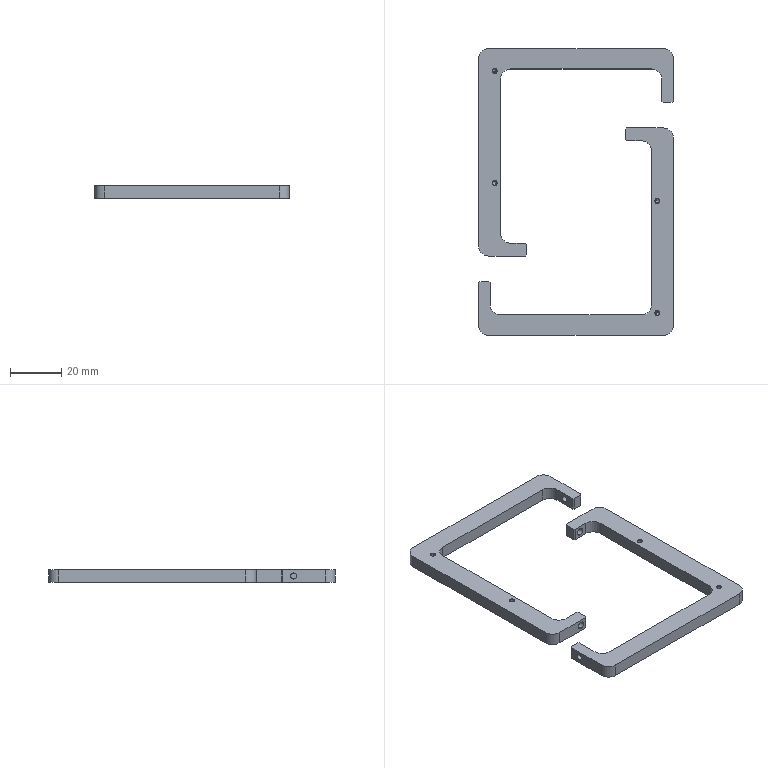NC program | NX | posted with a generic post | part box 76 x 112 x 5 mm
Whole program, first 1533 of 1825 lines:
N10 G17 G21 G94 G90
(DRILLING_1 , TOOL : CHAMFER_D4-90DEG)
N12 T03 M6
N14 G53
N16 G17 G0 G90 X-47.25 Y-31.75 B0. C0. S3000 M3
N18 G43 Z20. H3
N20 G94 G81 G99 Z-1.05 F200. R3.
N22 X-3.5
N24 X47.25 Y31.75
N26 X3.5
N28 G80
N30 G0 X3.5 Y31.75 Z20.
N32 M5
(DRILLING_1_COPY , TOOL : DRILL_D1.84-11-D3-40)
N34 T05 M6
N36 G53
N38 G17 G0 G90 X-47.25 Y-31.75 B0. C0. S3000 M3
N40 G43 Z20. H5
N42 G94 G83 G99 Z-4.6 F100. Q1. R3.
N44 X-3.5
N46 X47.25 Y31.75
N48 X3.5
N50 G80
N52 G0 X3.5 Y31.75 Z20.
N54 M5
(DRILLING_1_COPY_COPY , TOOL : FORM_M2-12-D3-39)
N56 T06 M6
N58 G53
N60 G17 G0 G90 X-47.25 Y-31.75 B0. C0. S300 M3
N62 G43 Z20. H6
N64 G84 G94 G99 Z-4.3 F120. R3.
N66 X-3.5
N68 X47.25 Y31.75
N70 X3.5
N72 G80
N74 G0 X3.5 Y31.75 Z20.
N76 M5
(FLOOR_WALL_1 , TOOL : D4_ROUGH)
N78 T01 M6
N80 G53
N82 G17 G0 G90 X-16.5 Y-24.5 B0. C0. S6500 M3
N84 G43 Z20. H1
N86 Z3.525
N88 G94 G1 Z0.525 F2000.
N90 Y-33.
N92 G3 X-15.5 Y-34. R1.
N94 G1 X21.
N96 Y-31.745
N98 X21.843 Y-29.642
N100 X21. Y-31.745
N102 G2 X16. Y-33.5 R8.
N104 G1 X-44.
N106 G2 X-52. Y-25.501 R8.
N108 G1 Y29.5
N110 Y-34.
N112 X-15.5
N114 Y-37.
N116 X21.
N118 G3 X24. Y-34. R3.
N120 G1 Y-20.2
N122 X21.
N124 Y-25.5
N126 G2 X16. Y-30.5 R5.
N128 G1 X-44.
N130 G2 X-49. Y-25.5 R5.
N132 G1 Y29.5
N134 X-52.
N136 G2 X-50.614 Y34. R8.
N138 G1 X-48.645 Y34.89
N140 X-50.614 Y34.
N142 X-52.
N144 Y29.5
N146 X-49.
N148 G2 X-44. Y34.5 R5.
N150 G1 X-36.
N152 Y37.
N154 X-52.
N156 G3 X-55. Y34. R3.
N158 G1 Y-34.
N160 G3 X-52. Y-37. R3.
N162 G1 X-15.5
N164 X-14.5
N166 G2 X-13.5 Y-38. R1.
N168 G1 Y-43.
N170 Z3.525
N172 G0 Z20.
N174 X-16.5 Y-24.5
N176 Z3.05
N178 G1 Z0.05
N180 Y-33.
N182 G3 X-15.5 Y-34. R1.
N184 G1 X21.
N186 Y-31.745
N188 X21.843 Y-29.642
N190 X21. Y-31.745
N192 G2 X16. Y-33.5 R8.
N194 G1 X-44.
N196 G2 X-52. Y-25.501 R8.
N198 G1 Y29.5
N200 Y-34.
N202 X-15.5
N204 Y-37.
N206 X21.
N208 G3 X24. Y-34. R3.
N210 G1 Y-20.2
N212 X21.
N214 Y-25.5
N216 G2 X16. Y-30.5 R5.
N218 G1 X-44.
N220 G2 X-49. Y-25.5 R5.
N222 G1 Y29.5
N224 X-52.
N226 G2 X-50.614 Y34. R8.
N228 G1 X-48.645 Y34.89
N230 X-50.614 Y34.
N232 X-52.
N234 Y29.5
N236 X-49.
N238 G2 X-44. Y34.5 R5.
N240 G1 X-36.
N242 Y37.
N244 X-52.
N246 G3 X-55. Y34. R3.
N248 G1 Y-34.
N250 G3 X-52. Y-37. R3.
N252 G1 X-15.5
N254 X-14.5
N256 G2 X-13.5 Y-38. R1.
N258 G1 Y-43.
N260 Z3.05
N262 G0 Z20.
N264 X16.5 Y24.5
N266 Z3.525
N268 G1 Z0.525
N270 Y33.
N272 G3 X15.5 Y34. R1.
N274 G1 X-21.
N276 Y31.745
N278 X-21.843 Y29.642
N280 X-21. Y31.745
N282 G2 X-16. Y33.5 R8.
N284 G1 X44.
N286 G2 X52. Y25.5 R8.
N288 G1 Y23.5
N290 G3 X53. Y23.768 R2.
N292 G1 Y-27.769
N294 G3 X51. Y-27.769 R2.
N296 G1 Y23.768
N298 G3 X52. Y23.5 R2.
N300 G1 Y25.5
N302 Y34.
N304 X15.5
N306 Y37.
N308 X-21.
N310 G3 X-24. Y34. R3.
N312 G1 Y20.2
N314 X-21.
N316 Y25.5
N318 G2 X-16. Y30.5 R5.
N320 G1 X44.
N322 G2 X49. Y25.5 R5.
N324 G1 Y-29.5
N326 X52. Y-29.501
N328 G2 X50.614 Y-34. R8.
N330 G1 X48.645 Y-34.89
N332 X50.614 Y-34.
N334 X52.
N336 Y-29.501
N338 X49. Y-29.5
N340 G2 X44. Y-34.5 R5.
N342 G1 X36.
N344 Y-37.
N346 X52.
N348 G3 X55. Y-34. R3.
N350 G1 Y34.
N352 G3 X52. Y37. R3.
N354 G1 X15.5
N356 X14.5
N358 G2 X13.5 Y38. R1.
N360 G1 Y43.
N362 Z3.525
N364 G0 Z20.
N366 X16.5 Y24.5
N368 Z3.05
N370 G1 Z0.05
N372 Y33.
N374 G3 X15.5 Y34. R1.
N376 G1 X-21.
N378 Y31.745
N380 X-21.843 Y29.642
N382 X-21. Y31.745
N384 G2 X-16. Y33.5 R8.
N386 G1 X44.
N388 G2 X52. Y25.5 R8.
N390 G1 Y23.5
N392 G3 X53. Y23.768 R2.
N394 G1 Y-27.769
N396 G3 X51. Y-27.769 R2.
N398 G1 Y23.768
N400 G3 X52. Y23.5 R2.
N402 G1 Y25.5
N404 Y34.
N406 X15.5
N408 Y37.
N410 X-21.
N412 G3 X-24. Y34. R3.
N414 G1 Y20.2
N416 X-21.
N418 Y25.5
N420 G2 X-16. Y30.5 R5.
N422 G1 X44.
N424 G2 X49. Y25.5 R5.
N426 G1 Y-29.5
N428 X52. Y-29.501
N430 G2 X50.614 Y-34. R8.
N432 G1 X48.645 Y-34.89
N434 X50.614 Y-34.
N436 X52.
N438 Y-29.501
N440 X49. Y-29.5
N442 G2 X44. Y-34.5 R5.
N444 G1 X36.
N446 Y-37.
N448 X52.
N450 G3 X55. Y-34. R3.
N452 G1 Y34.
N454 G3 X52. Y37. R3.
N456 G1 X15.5
N458 X14.5
N460 G2 X13.5 Y38. R1.
N462 G1 Y43.
N464 Z3.05
N466 G0 Z20.
N468 M5
(FLOOR_WALL_1_COPY , TOOL : D4-16-D4-75-3T)
N470 T02 M6
N472 G53
N474 G17 G0 G90 X-16.5 Y-24.5 B0. C0. S6500 M3
N476 G43 Z20. H2
N478 Z3.
N480 G94 G1 Z0. F800.
N482 Y-33.
N484 G3 X-15.5 Y-34. R1.
N486 G1 X21.
N488 Y-31.745
N490 X21.843 Y-29.642
N492 X21. Y-31.745
N494 G2 X16. Y-33.5 R8.
N496 G1 X-44.
N498 G2 X-52. Y-25.501 R8.
N500 G1 Y29.5
N502 Y-34.
N504 X-15.5
N506 Y-37.
N508 X21.
N510 G3 X24. Y-34. R3.
N512 G1 Y-20.2
N514 X21.
N516 Y-25.5
N518 G2 X16. Y-30.5 R5.
N520 G1 X-44.
N522 G2 X-49. Y-25.5 R5.
N524 G1 Y29.5
N526 X-52.
N528 G2 X-50.614 Y34. R8.
N530 G1 X-48.645 Y34.89
N532 X-50.614 Y34.
N534 X-52.
N536 Y29.5
N538 X-49.
N540 G2 X-44. Y34.5 R5.
N542 G1 X-36.
N544 Y37.
N546 X-52.
N548 G3 X-55. Y34. R3.
N550 G1 Y-34.
N552 G3 X-52. Y-37. R3.
N554 G1 X-15.5
N556 X-14.5
N558 G2 X-13.5 Y-38. R1.
N560 G1 Y-43.
N562 Z3.
N564 G0 Z20.
N566 X16.5 Y24.5
N568 Z3.
N570 G1 Z0.
N572 Y33.
N574 G3 X15.5 Y34. R1.
N576 G1 X-21.
N578 Y31.745
N580 X-21.843 Y29.642
N582 X-21. Y31.745
N584 G2 X-16. Y33.5 R8.
N586 G1 X44.
N588 G2 X52. Y25.5 R8.
N590 G1 Y23.5
N592 G3 X53. Y23.768 R2.
N594 G1 Y-27.769
N596 G3 X51. Y-27.769 R2.
N598 G1 Y23.768
N600 G3 X52. Y23.5 R2.
N602 G1 Y25.5
N604 Y34.
N606 X15.5
N608 Y37.
N610 X-21.
N612 G3 X-24. Y34. R3.
N614 G1 Y20.2
N616 X-21.
N618 Y25.5
N620 G2 X-16. Y30.5 R5.
N622 G1 X44.
N624 G2 X49. Y25.5 R5.
N626 G1 Y-29.5
N628 X52. Y-29.501
N630 G2 X50.614 Y-34. R8.
N632 G1 X48.645 Y-34.89
N634 X50.614 Y-34.
N636 X52.
N638 Y-29.501
N640 X49. Y-29.5
N642 G2 X44. Y-34.5 R5.
N644 G1 X36.
N646 Y-37.
N648 X52.
N650 G3 X55. Y-34. R3.
N652 G1 Y34.
N654 G3 X52. Y37. R3.
N656 G1 X15.5
N658 X14.5
N660 G2 X13.5 Y38. R1.
N662 G1 Y43.
N664 Z3.
N666 G0 Z20.
N668 M5
(PLANAR_MILL_2 , TOOL : D4_ROUGH)
N670 T01 M6
N672 G53
N674 G17 G0 G90 X-17.9 Y22.27 B0. C0. S6500 M3
N676 G43 Z20. H1
N678 Z1.
N680 G94 G1 Y19.344 Z0.996 F1500.
N682 X-18.263 Y18.467 Z0.995
N684 X-19.267 Y17.463 Z0.994
N686 X-20.144 Y17.1 Z0.992
N688 X-24.856 Z0.987
N690 X-25.733 Y17.463 Z0.985
N692 X-26.737 Y18.467 Z0.984
N694 X-27.1 Y19.344 Z0.983
N696 Y34.606 Z0.964
N698 X-26.707 Y36.237 Z0.962
N700 X-25.887 Y37.701 Z0.96
N702 X-24.701 Y38.887 Z0.958
N704 X-23.237 Y39.707 Z0.956
N706 X-21.606 Y40.1 Z0.954
N708 X52.606 Z0.863
N710 X54.237 Y39.707 Z0.861
N712 X55.701 Y38.887 Z0.859
N714 X56.887 Y37.701 Z0.857
N716 X57.707 Y36.237 Z0.855
N718 X58.1 Y34.606 Z0.853
N720 Y-34.606 Z0.768
N722 X57.707 Y-36.237 Z0.766
N724 X56.887 Y-37.701 Z0.764
N726 X55.701 Y-38.887 Z0.762
N728 X54.237 Y-39.707 Z0.76
N730 X52.606 Y-40.1 Z0.758
N732 X35.144 Z0.737
N734 X34.267 Y-39.737 Z0.735
N736 X33.263 Y-38.733 Z0.734
N738 X32.9 Y-37.856 Z0.733
N740 Y-33.644 Z0.727
N742 X33.263 Y-32.767 Z0.726
N744 X34.267 Y-31.763 Z0.725
N746 X35.144 Y-31.4 Z0.723
N748 X44.339 Z0.712
N750 X45.062 Y-31.112 Z0.711
N752 X45.612 Y-30.562 Z0.71
N754 X45.9 Y-29.839 Z0.709
N756 Y25.839 Z0.641
N758 X45.612 Y26.562 Z0.64
N760 X45.062 Y27.112 Z0.639
N762 X44.339 Y27.4 Z0.638
N764 X-16.339 Z0.564
N766 X-17.062 Y27.112 Z0.563
N768 X-17.612 Y26.562 Z0.562
N770 X-17.9 Y25.839 Z0.561
N772 Y19.344 Z0.553
N774 X-18.263 Y18.467 Z0.552
N776 X-19.267 Y17.463 Z0.551
N778 X-20.144 Y17.1 Z0.549
N780 X-24.856 Z0.544
N782 X-25.733 Y17.463 Z0.543
N784 X-26.737 Y18.467 Z0.541
N786 X-27.1 Y19.344 Z0.54
N788 Y34.606 Z0.521
N790 X-26.707 Y36.237 Z0.519
N792 X-25.887 Y37.701 Z0.517
N794 X-24.701 Y38.887 Z0.515
N796 X-23.237 Y39.707 Z0.513
N798 X-21.606 Y40.1 Z0.511
N800 X52.606 Z0.42
N802 X54.237 Y39.707 Z0.418
N804 X55.701 Y38.887 Z0.416
N806 X56.887 Y37.701 Z0.414
N808 X57.707 Y36.237 Z0.412
N810 X58.1 Y34.606 Z0.41
N812 Y-34.606 Z0.325
N814 X57.707 Y-36.237 Z0.323
N816 X56.887 Y-37.701 Z0.321
N818 X55.701 Y-38.887 Z0.319
N820 X54.237 Y-39.707 Z0.317
N822 X52.606 Y-40.1 Z0.315
N824 X35.144 Z0.294
N826 X34.267 Y-39.737 Z0.293
N828 X33.263 Y-38.733 Z0.291
N830 X32.9 Y-37.856 Z0.29
N832 Y-33.644 Z0.284
N834 X33.263 Y-32.767 Z0.283
N836 X34.267 Y-31.763 Z0.282
N838 X35.144 Y-31.4 Z0.28
N840 X44.339 Z0.269
N842 X45.062 Y-31.112 Z0.268
N844 X45.612 Y-30.562 Z0.267
N846 X45.9 Y-29.839 Z0.266
N848 Y25.839 Z0.198
N850 X45.612 Y26.562 Z0.197
N852 X45.062 Y27.112 Z0.196
N854 X44.339 Y27.4 Z0.195
N856 X-16.339 Z0.121
N858 X-17.062 Y27.112 Z0.12
N860 X-17.612 Y26.562 Z0.119
N862 X-17.9 Y25.839 Z0.118
N864 Y19.344 Z0.111
N866 X-18.263 Y18.467 Z0.109
N868 X-19.267 Y17.463 Z0.108
N870 X-20.144 Y17.1 Z0.106
N872 X-24.856 Z0.101
N874 X-25.733 Y17.463 Z0.1
N876 X-26.737 Y18.467 Z0.098
N878 X-27.1 Y19.344 Z0.097
N880 Y34.606 Z0.078
N882 X-26.707 Y36.237 Z0.076
N884 X-25.887 Y37.701 Z0.074
N886 X-24.701 Y38.887 Z0.072
N888 X-23.237 Y39.707 Z0.07
N890 X-21.606 Y40.1 Z0.068
N892 X52.606 Z-0.023
N894 X54.237 Y39.707 Z-0.025
N896 X55.701 Y38.887 Z-0.027
N898 X56.887 Y37.701 Z-0.029
N900 X57.707 Y36.237 Z-0.031
N902 X58.1 Y34.606 Z-0.033
N904 Y-34.606 Z-0.118
N906 X57.707 Y-36.237 Z-0.12
N908 X56.887 Y-37.701 Z-0.122
N910 X55.701 Y-38.887 Z-0.124
N912 X54.237 Y-39.707 Z-0.126
N914 X52.606 Y-40.1 Z-0.128
N916 X35.144 Z-0.149
N918 X34.267 Y-39.737 Z-0.15
N920 X33.263 Y-38.733 Z-0.152
N922 X32.9 Y-37.856 Z-0.153
N924 Y-33.644 Z-0.158
N926 X33.263 Y-32.767 Z-0.16
N928 X34.267 Y-31.763 Z-0.161
N930 X35.144 Y-31.4 Z-0.163
N932 X44.339 Z-0.174
N934 X45.062 Y-31.112 Z-0.175
N936 X45.612 Y-30.562 Z-0.176
N938 X45.9 Y-29.839 Z-0.177
N940 Y25.839 Z-0.245
N942 X45.612 Y26.562 Z-0.246
N944 X45.062 Y27.112 Z-0.247
N946 X44.339 Y27.4 Z-0.248
N948 X-16.339 Z-0.322
N950 X-17.062 Y27.112 Z-0.323
N952 X-17.612 Y26.562 Z-0.324
N954 X-17.9 Y25.839
N956 Y19.344 Z-0.332
N958 X-18.263 Y18.467 Z-0.334
N960 X-19.267 Y17.463 Z-0.335
N962 X-20.144 Y17.1 Z-0.336
N964 X-24.856 Z-0.342
N966 X-25.733 Y17.463 Z-0.343
N968 X-26.737 Y18.467 Z-0.345
N970 X-27.1 Y19.344 Z-0.346
N972 Y34.606 Z-0.365
N974 X-26.707 Y36.237 Z-0.367
N976 X-25.887 Y37.701 Z-0.369
N978 X-24.701 Y38.887 Z-0.371
N980 X-23.237 Y39.707 Z-0.373
N982 X-21.606 Y40.1 Z-0.375
N984 X52.606 Z-0.466
N986 X54.237 Y39.707 Z-0.468
N988 X55.701 Y38.887 Z-0.47
N990 X56.887 Y37.701 Z-0.472
N992 X57.707 Y36.237 Z-0.474
N994 X58.1 Y34.606 Z-0.476
N996 Y-34.606 Z-0.561
N998 X57.707 Y-36.237 Z-0.563
N1000 X56.887 Y-37.701 Z-0.565
N1002 X55.701 Y-38.887 Z-0.567
N1004 X54.237 Y-39.707 Z-0.569
N1006 X52.606 Y-40.1 Z-0.571
N1008 X35.144 Z-0.592
N1010 X34.267 Y-39.737 Z-0.593
N1012 X33.263 Y-38.733 Z-0.595
N1014 X32.9 Y-37.856 Z-0.596
N1016 Y-33.644 Z-0.601
N1018 X33.263 Y-32.767 Z-0.603
N1020 X34.267 Y-31.763 Z-0.604
N1022 X35.144 Y-31.4 Z-0.605
N1024 X44.339 Z-0.617
N1026 X45.062 Y-31.112 Z-0.618
N1028 X45.612 Y-30.562 Z-0.619
N1030 X45.9 Y-29.839 Z-0.62
N1032 Y25.839 Z-0.688
N1034 X45.612 Y26.562 Z-0.689
N1036 X45.062 Y27.112 Z-0.69
N1038 X44.339 Y27.4
N1040 X-16.339 Z-0.765
N1042 X-17.062 Y27.112 Z-0.766
N1044 X-17.612 Y26.562
N1046 X-17.9 Y25.839 Z-0.767
N1048 Y19.344 Z-0.775
N1050 X-18.263 Y18.467 Z-0.777
N1052 X-19.267 Y17.463 Z-0.778
N1054 X-20.144 Y17.1 Z-0.779
N1056 X-24.856 Z-0.785
N1058 X-25.733 Y17.463 Z-0.786
N1060 X-26.737 Y18.467 Z-0.788
N1062 X-27.1 Y19.344 Z-0.789
N1064 Y34.606 Z-0.808
N1066 X-26.707 Y36.237 Z-0.81
N1068 X-25.887 Y37.701 Z-0.812
N1070 X-24.701 Y38.887 Z-0.814
N1072 X-23.237 Y39.707 Z-0.816
N1074 X-21.606 Y40.1 Z-0.818
N1076 X52.606 Z-0.909
N1078 X54.237 Y39.707 Z-0.911
N1080 X55.701 Y38.887 Z-0.913
N1082 X56.887 Y37.701 Z-0.915
N1084 X57.707 Y36.237 Z-0.917
N1086 X58.1 Y34.606 Z-0.919
N1088 Y-34.606 Z-1.004
N1090 X57.707 Y-36.237 Z-1.006
N1092 X56.887 Y-37.701 Z-1.008
N1094 X55.701 Y-38.887 Z-1.01
N1096 X54.237 Y-39.707 Z-1.012
N1098 X52.606 Y-40.1 Z-1.014
N1100 X35.144 Z-1.035
N1102 X34.267 Y-39.737 Z-1.036
N1104 X33.263 Y-38.733 Z-1.038
N1106 X32.9 Y-37.856 Z-1.039
N1108 Y-33.644 Z-1.044
N1110 X33.263 Y-32.767 Z-1.046
N1112 X34.267 Y-31.763 Z-1.047
N1114 X35.144 Y-31.4 Z-1.048
N1116 X44.339 Z-1.06
N1118 X45.062 Y-31.112 Z-1.061
N1120 X45.612 Y-30.562 Z-1.062
N1122 X45.9 Y-29.839 Z-1.063
N1124 Y25.839 Z-1.131
N1126 X45.612 Y26.562
N1128 X45.062 Y27.112 Z-1.132
N1130 X44.339 Y27.4 Z-1.133
N1132 X-16.339 Z-1.208
N1134 X-17.062 Y27.112
N1136 X-17.612 Y26.562 Z-1.209
N1138 X-17.9 Y25.839 Z-1.21
N1140 Y19.344 Z-1.218
N1142 X-18.263 Y18.467 Z-1.219
N1144 X-19.267 Y17.463 Z-1.221
N1146 X-20.144 Y17.1 Z-1.222
N1148 X-24.856 Z-1.228
N1150 X-25.733 Y17.463 Z-1.229
N1152 X-26.737 Y18.467 Z-1.231
N1154 X-27.1 Y19.344 Z-1.232
N1156 Y34.606 Z-1.251
N1158 X-26.707 Y36.237 Z-1.253
N1160 X-25.887 Y37.701 Z-1.255
N1162 X-24.701 Y38.887 Z-1.257
N1164 X-23.237 Y39.707 Z-1.259
N1166 X-21.606 Y40.1 Z-1.261
N1168 X52.606 Z-1.352
N1170 X54.237 Y39.707 Z-1.354
N1172 X55.701 Y38.887 Z-1.356
N1174 X56.887 Y37.701 Z-1.358
N1176 X57.707 Y36.237 Z-1.36
N1178 X58.1 Y34.606 Z-1.362
N1180 Y-34.606 Z-1.447
N1182 X57.707 Y-36.237 Z-1.449
N1184 X56.887 Y-37.701 Z-1.451
N1186 X55.701 Y-38.887 Z-1.453
N1188 X54.237 Y-39.707 Z-1.455
N1190 X52.606 Y-40.1 Z-1.457
N1192 X35.144 Z-1.478
N1194 X34.267 Y-39.737 Z-1.479
N1196 X33.263 Y-38.733 Z-1.481
N1198 X32.9 Y-37.856 Z-1.482
N1200 Y-33.644 Z-1.487
N1202 X33.263 Y-32.767 Z-1.488
N1204 X34.267 Y-31.763 Z-1.49
N1206 X35.144 Y-31.4 Z-1.491
N1208 X44.339 Z-1.503
N1210 X45.062 Y-31.112 Z-1.504
N1212 X45.612 Y-30.562 Z-1.505
N1214 X45.9 Y-29.839
N1216 Y25.839 Z-1.573
N1218 X45.612 Y26.562 Z-1.574
N1220 X45.062 Y27.112 Z-1.575
N1222 X44.339 Y27.4 Z-1.576
N1224 X-16.339 Z-1.65
N1226 X-17.062 Y27.112 Z-1.651
N1228 X-17.612 Y26.562 Z-1.652
N1230 X-17.9 Y25.839 Z-1.653
N1232 Y19.344 Z-1.661
N1234 X-18.263 Y18.467 Z-1.662
N1236 X-19.267 Y17.463 Z-1.664
N1238 X-20.144 Y17.1 Z-1.665
N1240 X-24.856 Z-1.671
N1242 X-25.733 Y17.463 Z-1.672
N1244 X-26.737 Y18.467 Z-1.674
N1246 X-27.1 Y19.344 Z-1.675
N1248 Y34.606 Z-1.694
N1250 X-26.707 Y36.237 Z-1.696
N1252 X-25.887 Y37.701 Z-1.698
N1254 X-24.701 Y38.887 Z-1.7
N1256 X-23.237 Y39.707 Z-1.702
N1258 X-21.606 Y40.1 Z-1.704
N1260 X52.606 Z-1.795
N1262 X54.237 Y39.707 Z-1.797
N1264 X55.701 Y38.887 Z-1.799
N1266 X56.887 Y37.701 Z-1.801
N1268 X57.707 Y36.237 Z-1.803
N1270 X58.1 Y34.606 Z-1.805
N1272 Y-34.606 Z-1.89
N1274 X57.707 Y-36.237 Z-1.892
N1276 X56.887 Y-37.701 Z-1.894
N1278 X55.701 Y-38.887 Z-1.896
N1280 X54.237 Y-39.707 Z-1.898
N1282 X52.606 Y-40.1 Z-1.9
N1284 X35.144 Z-1.921
N1286 X34.267 Y-39.737 Z-1.922
N1288 X33.263 Y-38.733 Z-1.924
N1290 X32.9 Y-37.856 Z-1.925
N1292 Y-33.644 Z-1.93
N1294 X33.263 Y-32.767 Z-1.931
N1296 X34.267 Y-31.763 Z-1.933
N1298 X35.144 Y-31.4 Z-1.934
N1300 X44.339 Z-1.946
N1302 X45.062 Y-31.112 Z-1.947
N1304 X45.612 Y-30.562
N1306 X45.9 Y-29.839 Z-1.948
N1308 Y25.839 Z-2.016
N1310 X45.612 Y26.562 Z-2.017
N1312 X45.062 Y27.112 Z-2.018
N1314 X44.339 Y27.4 Z-2.019
N1316 X-16.339 Z-2.093
N1318 X-17.062 Y27.112 Z-2.094
N1320 X-17.612 Y26.562 Z-2.095
N1322 X-17.9 Y25.839 Z-2.096
N1324 Y19.344 Z-2.104
N1326 X-18.263 Y18.467 Z-2.105
N1328 X-19.267 Y17.463 Z-2.107
N1330 X-20.144 Y17.1 Z-2.108
N1332 X-24.856 Z-2.114
N1334 X-25.733 Y17.463 Z-2.115
N1336 X-26.737 Y18.467 Z-2.117
N1338 X-27.1 Y19.344 Z-2.118
N1340 Y34.606 Z-2.137
N1342 X-26.707 Y36.237 Z-2.139
N1344 X-25.887 Y37.701 Z-2.141
N1346 X-24.701 Y38.887 Z-2.143
N1348 X-23.237 Y39.707 Z-2.145
N1350 X-21.606 Y40.1 Z-2.147
N1352 X52.606 Z-2.238
N1354 X54.237 Y39.707 Z-2.24
N1356 X55.701 Y38.887 Z-2.242
N1358 X56.887 Y37.701 Z-2.244
N1360 X57.707 Y36.237 Z-2.246
N1362 X58.1 Y34.606 Z-2.248
N1364 Y-34.606 Z-2.332
N1366 X57.707 Y-36.237 Z-2.334
N1368 X56.887 Y-37.701 Z-2.337
N1370 X55.701 Y-38.887 Z-2.339
N1372 X54.237 Y-39.707 Z-2.341
N1374 X52.606 Y-40.1 Z-2.343
N1376 X35.144 Z-2.364
N1378 X34.267 Y-39.737 Z-2.365
N1380 X33.263 Y-38.733 Z-2.367
N1382 X32.9 Y-37.856 Z-2.368
N1384 Y-33.644 Z-2.373
N1386 X33.263 Y-32.767 Z-2.374
N1388 X34.267 Y-31.763 Z-2.376
N1390 X35.144 Y-31.4 Z-2.377
N1392 X44.339 Z-2.389
N1394 X45.062 Y-31.112
N1396 X45.612 Y-30.562 Z-2.39
N1398 X45.9 Y-29.839 Z-2.391
N1400 Y25.839 Z-2.459
N1402 X45.612 Y26.562 Z-2.46
N1404 X45.062 Y27.112 Z-2.461
N1406 X44.339 Y27.4 Z-2.462
N1408 X-16.339 Z-2.536
N1410 X-17.062 Y27.112 Z-2.537
N1412 X-17.612 Y26.562 Z-2.538
N1414 X-17.9 Y25.839 Z-2.539
N1416 Y19.344 Z-2.547
N1418 X-18.263 Y18.467 Z-2.548
N1420 X-19.267 Y17.463 Z-2.55
N1422 X-20.144 Y17.1 Z-2.551
N1424 X-24.856 Z-2.557
N1426 X-25.733 Y17.463 Z-2.558
N1428 X-26.737 Y18.467 Z-2.56
N1430 X-27.1 Y19.344 Z-2.561
N1432 Y34.606 Z-2.58
N1434 X-26.707 Y36.237 Z-2.582
N1436 X-25.887 Y37.701 Z-2.584
N1438 X-24.701 Y38.887 Z-2.586
N1440 X-23.237 Y39.707 Z-2.588
N1442 X-21.606 Y40.1 Z-2.59
N1444 X52.606 Z-2.681
N1446 X54.237 Y39.707 Z-2.683
N1448 X55.701 Y38.887 Z-2.685
N1450 X56.887 Y37.701 Z-2.687
N1452 X57.707 Y36.237 Z-2.689
N1454 X58.1 Y34.606 Z-2.691
N1456 Y-34.606 Z-2.775
N1458 X57.707 Y-36.237 Z-2.777
N1460 X56.887 Y-37.701 Z-2.779
N1462 X55.701 Y-38.887 Z-2.782
N1464 X54.237 Y-39.707 Z-2.784
N1466 X52.606 Y-40.1 Z-2.786
N1468 X35.144 Z-2.807
N1470 X34.267 Y-39.737 Z-2.808
N1472 X33.263 Y-38.733 Z-2.81
N1474 X32.9 Y-37.856 Z-2.811
N1476 Y-33.644 Z-2.816
N1478 X33.263 Y-32.767 Z-2.817
N1480 X34.267 Y-31.763 Z-2.819
N1482 X35.144 Y-31.4 Z-2.82
N1484 X44.339 Z-2.831
N1486 X45.062 Y-31.112 Z-2.832
N1488 X45.612 Y-30.562 Z-2.833
N1490 X45.9 Y-29.839 Z-2.834
N1492 Y25.839 Z-2.902
N1494 X45.612 Y26.562 Z-2.903
N1496 X45.062 Y27.112 Z-2.904
N1498 X44.339 Y27.4 Z-2.905
N1500 X-16.339 Z-2.979
N1502 X-17.062 Y27.112 Z-2.98
N1504 X-17.612 Y26.562 Z-2.981
N1506 X-17.9 Y25.839 Z-2.982
N1508 Y19.344 Z-2.99
N1510 X-18.263 Y18.467 Z-2.991
N1512 X-19.267 Y17.463 Z-2.993
N1514 X-20.144 Y17.1 Z-2.994
N1516 X-24.856 Z-3.
N1518 X-25.733 Y17.463 Z-3.001
N1520 X-26.737 Y18.467 Z-3.003
N1522 X-27.1 Y19.344 Z-3.004
N1524 Y34.606 Z-3.023
N1526 X-26.707 Y36.237 Z-3.025
N1528 X-25.887 Y37.701 Z-3.027
N1530 X-24.701 Y38.887 Z-3.029
N1532 X-23.237 Y39.707 Z-3.031
N1534 X-21.606 Y40.1 Z-3.033
N1536 X52.606 Z-3.124
N1538 X54.237 Y39.707 Z-3.126
N1540 X55.701 Y38.887 Z-3.128
N1542 X56.887 Y37.701 Z-3.13
N1544 X57.707 Y36.237 Z-3.132
N1546 X58.1 Y34.606 Z-3.134
N1548 Y-34.606 Z-3.218
N1550 X57.707 Y-36.237 Z-3.22
N1552 X56.887 Y-37.701 Z-3.222
N1554 X55.701 Y-38.887 Z-3.224
N1556 X54.237 Y-39.707 Z-3.227
N1558 X52.606 Y-40.1 Z-3.229
N1560 X35.144 Z-3.25
N1562 X34.267 Y-39.737 Z-3.251
N1564 X33.263 Y-38.733 Z-3.253
N1566 X32.9 Y-37.856 Z-3.254
N1568 Y-33.644 Z-3.259
N1570 X33.263 Y-32.767 Z-3.26
N1572 X34.267 Y-31.763 Z-3.262
N1574 X35.144 Y-31.4 Z-3.263
N1576 X44.339 Z-3.274
N1578 X45.062 Y-31.112 Z-3.275
N1580 X45.612 Y-30.562 Z-3.276
N1582 X45.9 Y-29.839 Z-3.277
N1584 Y25.839 Z-3.345
N1586 X45.612 Y26.562 Z-3.346
N1588 X45.062 Y27.112 Z-3.347
N1590 X44.339 Y27.4 Z-3.348
N1592 X-16.339 Z-3.422
N1594 X-17.062 Y27.112 Z-3.423
N1596 X-17.612 Y26.562 Z-3.424
N1598 X-17.9 Y25.839 Z-3.425
N1600 Y19.344 Z-3.433
N1602 X-18.263 Y18.467 Z-3.434
N1604 X-19.267 Y17.463 Z-3.436
N1606 X-20.144 Y17.1 Z-3.437
N1608 X-24.856 Z-3.443
N1610 X-25.733 Y17.463 Z-3.444
N1612 X-26.737 Y18.467 Z-3.446
N1614 X-27.1 Y19.344 Z-3.447
N1616 Y34.606 Z-3.466
N1618 X-26.707 Y36.237 Z-3.468
N1620 X-25.887 Y37.701 Z-3.47
N1622 X-24.701 Y38.887 Z-3.472
N1624 X-23.237 Y39.707 Z-3.474
N1626 X-21.606 Y40.1 Z-3.476
N1628 X52.606 Z-3.566
N1630 X54.237 Y39.707 Z-3.569
N1632 X55.701 Y38.887 Z-3.571
N1634 X56.887 Y37.701 Z-3.573
N1636 X57.707 Y36.237 Z-3.575
N1638 X58.1 Y34.606 Z-3.577
N1640 Y-34.606 Z-3.661
N1642 X57.707 Y-36.237 Z-3.663
N1644 X56.887 Y-37.701 Z-3.665
N1646 X55.701 Y-38.887 Z-3.667
N1648 X54.237 Y-39.707 Z-3.669
N1650 X52.606 Y-40.1 Z-3.672
N1652 X35.144 Z-3.693
N1654 X34.267 Y-39.737 Z-3.694
N1656 X33.263 Y-38.733 Z-3.696
N1658 X32.9 Y-37.856 Z-3.697
N1660 Y-33.644 Z-3.702
N1662 X33.263 Y-32.767 Z-3.703
N1664 X34.267 Y-31.763 Z-3.705
N1666 X35.144 Y-31.4 Z-3.706
N1668 X44.339 Z-3.717
N1670 X45.062 Y-31.112 Z-3.718
N1672 X45.612 Y-30.562 Z-3.719
N1674 X45.9 Y-29.839 Z-3.72
N1676 Y25.839 Z-3.788
N1678 X45.612 Y26.562 Z-3.789
N1680 X45.062 Y27.112 Z-3.79
N1682 X44.339 Y27.4 Z-3.791
N1684 X-16.339 Z-3.865
N1686 X-17.062 Y27.112 Z-3.866
N1688 X-17.612 Y26.562 Z-3.867
N1690 X-17.9 Y25.839 Z-3.868
N1692 Y19.344 Z-3.876
N1694 X-18.263 Y18.467 Z-3.877
N1696 X-19.267 Y17.463 Z-3.879
N1698 X-20.144 Y17.1 Z-3.88
N1700 X-24.856 Z-3.886
N1702 X-25.733 Y17.463 Z-3.887
N1704 X-26.737 Y18.467 Z-3.889
N1706 X-27.1 Y19.344 Z-3.89
N1708 Y34.606 Z-3.909
N1710 X-26.707 Y36.237 Z-3.911
N1712 X-25.887 Y37.701 Z-3.913
N1714 X-24.701 Y38.887 Z-3.915
N1716 X-23.237 Y39.707 Z-3.917
N1718 X-21.606 Y40.1 Z-3.919
N1720 X52.606 Z-4.009
N1722 X54.237 Y39.707 Z-4.011
N1724 X55.701 Y38.887 Z-4.014
N1726 X56.887 Y37.701 Z-4.016
N1728 X57.707 Y36.237 Z-4.018
N1730 X58.1 Y34.606 Z-4.02
N1732 Y-34.606 Z-4.104
N1734 X57.707 Y-36.237 Z-4.106
N1736 X56.887 Y-37.701 Z-4.108
N1738 X55.701 Y-38.887 Z-4.11
N1740 X54.237 Y-39.707 Z-4.112
N1742 X52.606 Y-40.1 Z-4.114
N1744 X35.144 Z-4.136
N1746 X34.267 Y-39.737 Z-4.137
N1748 X33.263 Y-38.733 Z-4.139
N1750 X32.9 Y-37.856 Z-4.14
N1752 Y-33.644 Z-4.145
N1754 X33.263 Y-32.767 Z-4.146
N1756 X34.267 Y-31.763 Z-4.148
N1758 X35.144 Y-31.4 Z-4.149
N1760 X44.339 Z-4.16
N1762 X45.062 Y-31.112 Z-4.161
N1764 X45.612 Y-30.562 Z-4.162
N1766 X45.9 Y-29.839 Z-4.163
N1768 Y25.839 Z-4.231
N1770 X45.612 Y26.562 Z-4.232
N1772 X45.062 Y27.112 Z-4.233
N1774 X44.339 Y27.4 Z-4.234
N1776 X-16.339 Z-4.308
N1778 X-17.062 Y27.112 Z-4.309
N1780 X-17.612 Y26.562 Z-4.31
N1782 X-17.9 Y25.839 Z-4.311
N1784 Y19.344 Z-4.319
N1786 X-18.263 Y18.467 Z-4.32
N1788 X-19.267 Y17.463 Z-4.322
N1790 X-20.144 Y17.1 Z-4.323
N1792 X-24.856 Z-4.329
N1794 X-25.733 Y17.463 Z-4.33
N1796 X-26.737 Y18.467 Z-4.332
N1798 X-27.1 Y19.344 Z-4.333
N1800 Y34.606 Z-4.351
N1802 X-26.707 Y36.237 Z-4.354
N1804 X-25.887 Y37.701 Z-4.356
N1806 X-24.701 Y38.887 Z-4.358
N1808 X-23.237 Y39.707 Z-4.36
N1810 X-21.606 Y40.1 Z-4.362
N1812 X52.606 Z-4.452
N1814 X54.237 Y39.707 Z-4.454
N1816 X55.701 Y38.887 Z-4.456
N1818 X56.887 Y37.701 Z-4.459
N1820 X57.707 Y36.237 Z-4.461
N1822 X58.1 Y34.606 Z-4.463
N1824 Y-34.606 Z-4.547
N1826 X57.707 Y-36.237 Z-4.549
N1828 X56.887 Y-37.701 Z-4.551
N1830 X55.701 Y-38.887 Z-4.553
N1832 X54.237 Y-39.707 Z-4.555
N1834 X52.606 Y-40.1 Z-4.557
N1836 X35.144 Z-4.579
N1838 X34.267 Y-39.737 Z-4.58
N1840 X33.263 Y-38.733 Z-4.582
N1842 X32.9 Y-37.856 Z-4.583
N1844 Y-33.644 Z-4.588
N1846 X33.263 Y-32.767 Z-4.589
N1848 X34.267 Y-31.763 Z-4.591
N1850 X35.144 Y-31.4 Z-4.592
N1852 X44.339 Z-4.603
N1854 X45.062 Y-31.112 Z-4.604
N1856 X45.612 Y-30.562 Z-4.605
N1858 X45.9 Y-29.839 Z-4.606
N1860 Y25.839 Z-4.674
N1862 X45.612 Y26.562 Z-4.675
N1864 X45.062 Y27.112 Z-4.676
N1866 X44.339 Y27.4 Z-4.677
N1868 X-16.339 Z-4.751
N1870 X-17.062 Y27.112 Z-4.752
N1872 X-17.612 Y26.562 Z-4.753
N1874 X-17.9 Y25.839 Z-4.754
N1876 Y19.344 Z-4.762
N1878 X-18.263 Y18.467 Z-4.763
N1880 X-19.267 Y17.463 Z-4.765
N1882 X-20.144 Y17.1 Z-4.766
N1884 X-24.856 Z-4.772
N1886 X-25.733 Y17.463 Z-4.773
N1888 X-26.737 Y18.467 Z-4.775
N1890 X-27.1 Y19.344 Z-4.776
N1892 Y34.606 Z-4.794
N1894 X-26.707 Y36.237 Z-4.796
N1896 X-25.887 Y37.701 Z-4.799
N1898 X-24.701 Y38.887 Z-4.801
N1900 X-23.237 Y39.707 Z-4.803
N1902 X-21.606 Y40.1 Z-4.805
N1904 X15.5 Z-4.85
N1906 X52.
N1908 G2 X58.1 Y34. R6.1
N1910 G1 Y-34.
N1912 G2 X52. Y-40.1 R6.1
N1914 G1 X35.5
N1916 G2 X34.015 Y-39.485 R2.1
N1918 G1 X33.515 Y-38.985
N1920 G2 X32.9 Y-37.5 R2.1
N1922 G1 Y-34.
N1924 G2 X33.515 Y-32.515 R2.1
N1926 G1 X34.015 Y-32.015
N1928 G2 X35.5 Y-31.4 R2.1
N1930 G1 X44.
N1932 G3 X45.9 Y-29.5 R1.9
N1934 G1 Y25.5
N1936 G3 X44. Y27.4 R1.9
N1938 G1 X-16.
N1940 G3 X-17.9 Y25.5 R1.9
N1942 G1 Y19.7
N1944 G2 X-18.515 Y18.215 R2.1
N1946 G1 X-19.015 Y17.715
N1948 G2 X-20.5 Y17.1 R2.1
N1950 G1 X-24.5
N1952 G2 X-25.985 Y17.715 R2.1
N1954 G1 X-26.485 Y18.215
N1956 G2 X-27.1 Y19.7 R2.1
N1958 G1 Y34.
N1960 G2 X-21. Y40.1 R6.1
N1962 G1 X15.5
N1964 Z-3.85
N1966 G0 Z20.
N1968 X17.9 Y-22.27
N1970 Z1.
N1972 G1 Y-19.344 Z0.996
N1974 X18.263 Y-18.467 Z0.995
N1976 X19.267 Y-17.463 Z0.994
N1978 X20.144 Y-17.1 Z0.992
N1980 X24.856 Z0.987
N1982 X25.733 Y-17.463 Z0.985
N1984 X26.737 Y-18.467 Z0.984
N1986 X27.1 Y-19.344 Z0.983
N1988 Y-34.606 Z0.964
N1990 X26.707 Y-36.237 Z0.962
N1992 X25.887 Y-37.701 Z0.96
N1994 X24.701 Y-38.887 Z0.958
N1996 X23.237 Y-39.707 Z0.956
N1998 X21.606 Y-40.1 Z0.954
N2000 X-52.606 Z0.863
N2002 X-54.237 Y-39.707 Z0.861
N2004 X-55.701 Y-38.887 Z0.859
N2006 X-56.887 Y-37.701 Z0.857
N2008 X-57.707 Y-36.237 Z0.855
N2010 X-58.1 Y-34.606 Z0.853
N2012 Y34.606 Z0.768
N2014 X-57.707 Y36.237 Z0.766
N2016 X-56.887 Y37.701 Z0.764
N2018 X-55.701 Y38.887 Z0.762
N2020 X-54.237 Y39.707 Z0.76
N2022 X-52.606 Y40.1 Z0.758
N2024 X-35.144 Z0.737
N2026 X-34.267 Y39.737 Z0.735
N2028 X-33.263 Y38.733 Z0.734
N2030 X-32.9 Y37.856 Z0.733
N2032 Y33.644 Z0.727
N2034 X-33.263 Y32.767 Z0.726
N2036 X-34.267 Y31.763 Z0.725
N2038 X-35.144 Y31.4 Z0.723
N2040 X-44.339 Z0.712
N2042 X-45.062 Y31.112 Z0.711
N2044 X-45.612 Y30.562 Z0.71
N2046 X-45.9 Y29.839 Z0.709
N2048 Y-25.839 Z0.641
N2050 X-45.612 Y-26.562 Z0.64
N2052 X-45.062 Y-27.112 Z0.639
N2054 X-44.339 Y-27.4 Z0.638
N2056 X16.339 Z0.564
N2058 X17.062 Y-27.112 Z0.563
N2060 X17.612 Y-26.562 Z0.562
N2062 X17.9 Y-25.839 Z0.561
N2064 Y-19.344 Z0.553
N2066 X18.263 Y-18.467 Z0.552
N2068 X19.267 Y-17.463 Z0.551
N2070 X20.144 Y-17.1 Z0.549
N2072 X24.856 Z0.544
N2074 X25.733 Y-17.463 Z0.543
N2076 X26.737 Y-18.467 Z0.541
N2078 X27.1 Y-19.344 Z0.54
N2080 Y-34.606 Z0.521
N2082 X26.707 Y-36.237 Z0.519
N2084 X25.887 Y-37.701 Z0.517
N2086 X24.701 Y-38.887 Z0.515
N2088 X23.237 Y-39.707 Z0.513
N2090 X21.606 Y-40.1 Z0.511
N2092 X-52.606 Z0.42
N2094 X-54.237 Y-39.707 Z0.418
N2096 X-55.701 Y-38.887 Z0.416
N2098 X-56.887 Y-37.701 Z0.414
N2100 X-57.707 Y-36.237 Z0.412
N2102 X-58.1 Y-34.606 Z0.41
N2104 Y34.606 Z0.325
N2106 X-57.707 Y36.237 Z0.323
N2108 X-56.887 Y37.701 Z0.321
N2110 X-55.701 Y38.887 Z0.319
N2112 X-54.237 Y39.707 Z0.317
N2114 X-52.606 Y40.1 Z0.315
N2116 X-35.144 Z0.294
N2118 X-34.267 Y39.737 Z0.293
N2120 X-33.263 Y38.733 Z0.291
N2122 X-32.9 Y37.856 Z0.29
N2124 Y33.644 Z0.284
N2126 X-33.263 Y32.767 Z0.283
N2128 X-34.267 Y31.763 Z0.282
N2130 X-35.144 Y31.4 Z0.28
N2132 X-44.339 Z0.269
N2134 X-45.062 Y31.112 Z0.268
N2136 X-45.612 Y30.562 Z0.267
N2138 X-45.9 Y29.839 Z0.266
N2140 Y-25.839 Z0.198
N2142 X-45.612 Y-26.562 Z0.197
N2144 X-45.062 Y-27.112 Z0.196
N2146 X-44.339 Y-27.4 Z0.195
N2148 X16.339 Z0.121
N2150 X17.062 Y-27.112 Z0.12
N2152 X17.612 Y-26.562 Z0.119
N2154 X17.9 Y-25.839 Z0.118
N2156 Y-19.344 Z0.111
N2158 X18.263 Y-18.467 Z0.109
N2160 X19.267 Y-17.463 Z0.108
N2162 X20.144 Y-17.1 Z0.106
N2164 X24.856 Z0.101
N2166 X25.733 Y-17.463 Z0.1
N2168 X26.737 Y-18.467 Z0.098
N2170 X27.1 Y-19.344 Z0.097
N2172 Y-34.606 Z0.078
N2174 X26.707 Y-36.237 Z0.076
N2176 X25.887 Y-37.701 Z0.074
N2178 X24.701 Y-38.887 Z0.072
N2180 X23.237 Y-39.707 Z0.07
N2182 X21.606 Y-40.1 Z0.068
N2184 X-52.606 Z-0.023
N2186 X-54.237 Y-39.707 Z-0.025
N2188 X-55.701 Y-38.887 Z-0.027
N2190 X-56.887 Y-37.701 Z-0.029
N2192 X-57.707 Y-36.237 Z-0.031
N2194 X-58.1 Y-34.606 Z-0.033
N2196 Y34.606 Z-0.118
N2198 X-57.707 Y36.237 Z-0.12
N2200 X-56.887 Y37.701 Z-0.122
N2202 X-55.701 Y38.887 Z-0.124
N2204 X-54.237 Y39.707 Z-0.126
N2206 X-52.606 Y40.1 Z-0.128
N2208 X-35.144 Z-0.149
N2210 X-34.267 Y39.737 Z-0.15
N2212 X-33.263 Y38.733 Z-0.152
N2214 X-32.9 Y37.856 Z-0.153
N2216 Y33.644 Z-0.158
N2218 X-33.263 Y32.767 Z-0.16
N2220 X-34.267 Y31.763 Z-0.161
N2222 X-35.144 Y31.4 Z-0.163
N2224 X-44.339 Z-0.174
N2226 X-45.062 Y31.112 Z-0.175
N2228 X-45.612 Y30.562 Z-0.176
N2230 X-45.9 Y29.839 Z-0.177
N2232 Y-25.839 Z-0.245
N2234 X-45.612 Y-26.562 Z-0.246
N2236 X-45.062 Y-27.112 Z-0.247
N2238 X-44.339 Y-27.4 Z-0.248
N2240 X16.339 Z-0.322
N2242 X17.062 Y-27.112 Z-0.323
N2244 X17.612 Y-26.562 Z-0.324
N2246 X17.9 Y-25.839
N2248 Y-19.344 Z-0.332
N2250 X18.263 Y-18.467 Z-0.334
N2252 X19.267 Y-17.463 Z-0.335
N2254 X20.144 Y-17.1 Z-0.336
N2256 X24.856 Z-0.342
N2258 X25.733 Y-17.463 Z-0.343
N2260 X26.737 Y-18.467 Z-0.345
N2262 X27.1 Y-19.344 Z-0.346
N2264 Y-34.606 Z-0.365
N2266 X26.707 Y-36.237 Z-0.367
N2268 X25.887 Y-37.701 Z-0.369
N2270 X24.701 Y-38.887 Z-0.371
N2272 X23.237 Y-39.707 Z-0.373
N2274 X21.606 Y-40.1 Z-0.375
N2276 X-52.606 Z-0.466
N2278 X-54.237 Y-39.707 Z-0.468
N2280 X-55.701 Y-38.887 Z-0.47
N2282 X-56.887 Y-37.701 Z-0.472
N2284 X-57.707 Y-36.237 Z-0.474
N2286 X-58.1 Y-34.606 Z-0.476
N2288 Y34.606 Z-0.561
N2290 X-57.707 Y36.237 Z-0.563
N2292 X-56.887 Y37.701 Z-0.565
N2294 X-55.701 Y38.887 Z-0.567
N2296 X-54.237 Y39.707 Z-0.569
N2298 X-52.606 Y40.1 Z-0.571
N2300 X-35.144 Z-0.592
N2302 X-34.267 Y39.737 Z-0.593
N2304 X-33.263 Y38.733 Z-0.595
N2306 X-32.9 Y37.856 Z-0.596
N2308 Y33.644 Z-0.601
N2310 X-33.263 Y32.767 Z-0.603
N2312 X-34.267 Y31.763 Z-0.604
N2314 X-35.144 Y31.4 Z-0.605
N2316 X-44.339 Z-0.617
N2318 X-45.062 Y31.112 Z-0.618
N2320 X-45.612 Y30.562 Z-0.619
N2322 X-45.9 Y29.839 Z-0.62
N2324 Y-25.839 Z-0.688
N2326 X-45.612 Y-26.562 Z-0.689
N2328 X-45.062 Y-27.112 Z-0.69
N2330 X-44.339 Y-27.4
N2332 X16.339 Z-0.765
N2334 X17.062 Y-27.112 Z-0.766
N2336 X17.612 Y-26.562
N2338 X17.9 Y-25.839 Z-0.767
N2340 Y-19.344 Z-0.775
N2342 X18.263 Y-18.467 Z-0.777
N2344 X19.267 Y-17.463 Z-0.778
N2346 X20.144 Y-17.1 Z-0.779
N2348 X24.856 Z-0.785
N2350 X25.733 Y-17.463 Z-0.786
N2352 X26.737 Y-18.467 Z-0.788
N2354 X27.1 Y-19.344 Z-0.789
N2356 Y-34.606 Z-0.808
N2358 X26.707 Y-36.237 Z-0.81
N2360 X25.887 Y-37.701 Z-0.812
N2362 X24.701 Y-38.887 Z-0.814
N2364 X23.237 Y-39.707 Z-0.816
N2366 X21.606 Y-40.1 Z-0.818
N2368 X-52.606 Z-0.909
N2370 X-54.237 Y-39.707 Z-0.911
N2372 X-55.701 Y-38.887 Z-0.913
N2374 X-56.887 Y-37.701 Z-0.915
N2376 X-57.707 Y-36.237 Z-0.917
N2378 X-58.1 Y-34.606 Z-0.919
N2380 Y34.606 Z-1.004
N2382 X-57.707 Y36.237 Z-1.006
N2384 X-56.887 Y37.701 Z-1.008
N2386 X-55.701 Y38.887 Z-1.01
N2388 X-54.237 Y39.707 Z-1.012
N2390 X-52.606 Y40.1 Z-1.014
N2392 X-35.144 Z-1.035
N2394 X-34.267 Y39.737 Z-1.036
N2396 X-33.263 Y38.733 Z-1.038
N2398 X-32.9 Y37.856 Z-1.039
N2400 Y33.644 Z-1.044
N2402 X-33.263 Y32.767 Z-1.046
N2404 X-34.267 Y31.763 Z-1.047
N2406 X-35.144 Y31.4 Z-1.048
N2408 X-44.339 Z-1.06
N2410 X-45.062 Y31.112 Z-1.061
N2412 X-45.612 Y30.562 Z-1.062
N2414 X-45.9 Y29.839 Z-1.063
N2416 Y-25.839 Z-1.131
N2418 X-45.612 Y-26.562
N2420 X-45.062 Y-27.112 Z-1.132
N2422 X-44.339 Y-27.4 Z-1.133
N2424 X16.339 Z-1.208
N2426 X17.062 Y-27.112
N2428 X17.612 Y-26.562 Z-1.209
N2430 X17.9 Y-25.839 Z-1.21
N2432 Y-19.344 Z-1.218
N2434 X18.263 Y-18.467 Z-1.219
N2436 X19.267 Y-17.463 Z-1.221
N2438 X20.144 Y-17.1 Z-1.222
N2440 X24.856 Z-1.228
N2442 X25.733 Y-17.463 Z-1.229
N2444 X26.737 Y-18.467 Z-1.231
N2446 X27.1 Y-19.344 Z-1.232
N2448 Y-34.606 Z-1.251
N2450 X26.707 Y-36.237 Z-1.253
N2452 X25.887 Y-37.701 Z-1.255
N2454 X24.701 Y-38.887 Z-1.257
N2456 X23.237 Y-39.707 Z-1.259
N2458 X21.606 Y-40.1 Z-1.261
N2460 X-52.606 Z-1.352
N2462 X-54.237 Y-39.707 Z-1.354
N2464 X-55.701 Y-38.887 Z-1.356
N2466 X-56.887 Y-37.701 Z-1.358
N2468 X-57.707 Y-36.237 Z-1.36
N2470 X-58.1 Y-34.606 Z-1.362
N2472 Y34.606 Z-1.447
N2474 X-57.707 Y36.237 Z-1.449
N2476 X-56.887 Y37.701 Z-1.451
N2478 X-55.701 Y38.887 Z-1.453
N2480 X-54.237 Y39.707 Z-1.455
N2482 X-52.606 Y40.1 Z-1.457
N2484 X-35.144 Z-1.478
N2486 X-34.267 Y39.737 Z-1.479
N2488 X-33.263 Y38.733 Z-1.481
N2490 X-32.9 Y37.856 Z-1.482
N2492 Y33.644 Z-1.487
N2494 X-33.263 Y32.767 Z-1.488
N2496 X-34.267 Y31.763 Z-1.49
N2498 X-35.144 Y31.4 Z-1.491
N2500 X-44.339 Z-1.503
N2502 X-45.062 Y31.112 Z-1.504
N2504 X-45.612 Y30.562 Z-1.505
N2506 X-45.9 Y29.839
N2508 Y-25.839 Z-1.573
N2510 X-45.612 Y-26.562 Z-1.574
N2512 X-45.062 Y-27.112 Z-1.575
N2514 X-44.339 Y-27.4 Z-1.576
N2516 X16.339 Z-1.65
N2518 X17.062 Y-27.112 Z-1.651
N2520 X17.612 Y-26.562 Z-1.652
N2522 X17.9 Y-25.839 Z-1.653
N2524 Y-19.344 Z-1.661
N2526 X18.263 Y-18.467 Z-1.662
N2528 X19.267 Y-17.463 Z-1.664
N2530 X20.144 Y-17.1 Z-1.665
N2532 X24.856 Z-1.671
N2534 X25.733 Y-17.463 Z-1.672
N2536 X26.737 Y-18.467 Z-1.674
N2538 X27.1 Y-19.344 Z-1.675
N2540 Y-34.606 Z-1.694
N2542 X26.707 Y-36.237 Z-1.696
N2544 X25.887 Y-37.701 Z-1.698
N2546 X24.701 Y-38.887 Z-1.7
N2548 X23.237 Y-39.707 Z-1.702
N2550 X21.606 Y-40.1 Z-1.704
N2552 X-52.606 Z-1.795
N2554 X-54.237 Y-39.707 Z-1.797
N2556 X-55.701 Y-38.887 Z-1.799
N2558 X-56.887 Y-37.701 Z-1.801
N2560 X-57.707 Y-36.237 Z-1.803
N2562 X-58.1 Y-34.606 Z-1.805
N2564 Y34.606 Z-1.89
N2566 X-57.707 Y36.237 Z-1.892
N2568 X-56.887 Y37.701 Z-1.894
N2570 X-55.701 Y38.887 Z-1.896
N2572 X-54.237 Y39.707 Z-1.898
N2574 X-52.606 Y40.1 Z-1.9
N2576 X-35.144 Z-1.921
N2578 X-34.267 Y39.737 Z-1.922
N2580 X-33.263 Y38.733 Z-1.924
N2582 X-32.9 Y37.856 Z-1.925
N2584 Y33.644 Z-1.93
N2586 X-33.263 Y32.767 Z-1.931
N2588 X-34.267 Y31.763 Z-1.933
N2590 X-35.144 Y31.4 Z-1.934
N2592 X-44.339 Z-1.946
N2594 X-45.062 Y31.112 Z-1.947
N2596 X-45.612 Y30.562
N2598 X-45.9 Y29.839 Z-1.948
N2600 Y-25.839 Z-2.016
N2602 X-45.612 Y-26.562 Z-2.017
N2604 X-45.062 Y-27.112 Z-2.018
N2606 X-44.339 Y-27.4 Z-2.019
N2608 X16.339 Z-2.093
N2610 X17.062 Y-27.112 Z-2.094
N2612 X17.612 Y-26.562 Z-2.095
N2614 X17.9 Y-25.839 Z-2.096
N2616 Y-19.344 Z-2.104
N2618 X18.263 Y-18.467 Z-2.105
N2620 X19.267 Y-17.463 Z-2.107
N2622 X20.144 Y-17.1 Z-2.108
N2624 X24.856 Z-2.114
N2626 X25.733 Y-17.463 Z-2.115
N2628 X26.737 Y-18.467 Z-2.117
N2630 X27.1 Y-19.344 Z-2.118
N2632 Y-34.606 Z-2.137
N2634 X26.707 Y-36.237 Z-2.139
N2636 X25.887 Y-37.701 Z-2.141
N2638 X24.701 Y-38.887 Z-2.143
N2640 X23.237 Y-39.707 Z-2.145
N2642 X21.606 Y-40.1 Z-2.147
N2644 X-52.606 Z-2.238
N2646 X-54.237 Y-39.707 Z-2.24
N2648 X-55.701 Y-38.887 Z-2.242
N2650 X-56.887 Y-37.701 Z-2.244
N2652 X-57.707 Y-36.237 Z-2.246
N2654 X-58.1 Y-34.606 Z-2.248
N2656 Y34.606 Z-2.332
N2658 X-57.707 Y36.237 Z-2.334
N2660 X-56.887 Y37.701 Z-2.337
N2662 X-55.701 Y38.887 Z-2.339
N2664 X-54.237 Y39.707 Z-2.341
N2666 X-52.606 Y40.1 Z-2.343
N2668 X-35.144 Z-2.364
N2670 X-34.267 Y39.737 Z-2.365
N2672 X-33.263 Y38.733 Z-2.367
N2674 X-32.9 Y37.856 Z-2.368
N2676 Y33.644 Z-2.373
N2678 X-33.263 Y32.767 Z-2.374
N2680 X-34.267 Y31.763 Z-2.376
N2682 X-35.144 Y31.4 Z-2.377
N2684 X-44.339 Z-2.389
N2686 X-45.062 Y31.112
N2688 X-45.612 Y30.562 Z-2.39
N2690 X-45.9 Y29.839 Z-2.391
N2692 Y-25.839 Z-2.459
N2694 X-45.612 Y-26.562 Z-2.46
N2696 X-45.062 Y-27.112 Z-2.461
N2698 X-44.339 Y-27.4 Z-2.462
N2700 X16.339 Z-2.536
N2702 X17.062 Y-27.112 Z-2.537
N2704 X17.612 Y-26.562 Z-2.538
N2706 X17.9 Y-25.839 Z-2.539
N2708 Y-19.344 Z-2.547
N2710 X18.263 Y-18.467 Z-2.548
N2712 X19.267 Y-17.463 Z-2.55
N2714 X20.144 Y-17.1 Z-2.551
N2716 X24.856 Z-2.557
N2718 X25.733 Y-17.463 Z-2.558
N2720 X26.737 Y-18.467 Z-2.56
N2722 X27.1 Y-19.344 Z-2.561
N2724 Y-34.606 Z-2.58
N2726 X26.707 Y-36.237 Z-2.582
N2728 X25.887 Y-37.701 Z-2.584
N2730 X24.701 Y-38.887 Z-2.586
N2732 X23.237 Y-39.707 Z-2.588
N2734 X21.606 Y-40.1 Z-2.59
N2736 X-52.606 Z-2.681
N2738 X-54.237 Y-39.707 Z-2.683
N2740 X-55.701 Y-38.887 Z-2.685
N2742 X-56.887 Y-37.701 Z-2.687
N2744 X-57.707 Y-36.237 Z-2.689
N2746 X-58.1 Y-34.606 Z-2.691
N2748 Y34.606 Z-2.775
N2750 X-57.707 Y36.237 Z-2.777
N2752 X-56.887 Y37.701 Z-2.779
N2754 X-55.701 Y38.887 Z-2.782
N2756 X-54.237 Y39.707 Z-2.784
N2758 X-52.606 Y40.1 Z-2.786
N2760 X-35.144 Z-2.807
N2762 X-34.267 Y39.737 Z-2.808
N2764 X-33.263 Y38.733 Z-2.81
N2766 X-32.9 Y37.856 Z-2.811
N2768 Y33.644 Z-2.816
N2770 X-33.263 Y32.767 Z-2.817
N2772 X-34.267 Y31.763 Z-2.819
N2774 X-35.144 Y31.4 Z-2.82
N2776 X-44.339 Z-2.831
N2778 X-45.062 Y31.112 Z-2.832
N2780 X-45.612 Y30.562 Z-2.833
N2782 X-45.9 Y29.839 Z-2.834
N2784 Y-25.839 Z-2.902
N2786 X-45.612 Y-26.562 Z-2.903
N2788 X-45.062 Y-27.112 Z-2.904
N2790 X-44.339 Y-27.4 Z-2.905
N2792 X16.339 Z-2.979
N2794 X17.062 Y-27.112 Z-2.98
N2796 X17.612 Y-26.562 Z-2.981
N2798 X17.9 Y-25.839 Z-2.982
N2800 Y-19.344 Z-2.99
N2802 X18.263 Y-18.467 Z-2.991
N2804 X19.267 Y-17.463 Z-2.993
N2806 X20.144 Y-17.1 Z-2.994
N2808 X24.856 Z-3.
N2810 X25.733 Y-17.463 Z-3.001
N2812 X26.737 Y-18.467 Z-3.003
N2814 X27.1 Y-19.344 Z-3.004
N2816 Y-34.606 Z-3.023
N2818 X26.707 Y-36.237 Z-3.025
N2820 X25.887 Y-37.701 Z-3.027
N2822 X24.701 Y-38.887 Z-3.029
N2824 X23.237 Y-39.707 Z-3.031
N2826 X21.606 Y-40.1 Z-3.033
N2828 X-52.606 Z-3.124
N2830 X-54.237 Y-39.707 Z-3.126
N2832 X-55.701 Y-38.887 Z-3.128
N2834 X-56.887 Y-37.701 Z-3.13
N2836 X-57.707 Y-36.237 Z-3.132
N2838 X-58.1 Y-34.606 Z-3.134
N2840 Y34.606 Z-3.218
N2842 X-57.707 Y36.237 Z-3.22
N2844 X-56.887 Y37.701 Z-3.222
N2846 X-55.701 Y38.887 Z-3.224
N2848 X-54.237 Y39.707 Z-3.227
N2850 X-52.606 Y40.1 Z-3.229
N2852 X-35.144 Z-3.25
N2854 X-34.267 Y39.737 Z-3.251
N2856 X-33.263 Y38.733 Z-3.253
N2858 X-32.9 Y37.856 Z-3.254
N2860 Y33.644 Z-3.259
N2862 X-33.263 Y32.767 Z-3.26
N2864 X-34.267 Y31.763 Z-3.262
N2866 X-35.144 Y31.4 Z-3.263
N2868 X-44.339 Z-3.274
N2870 X-45.062 Y31.112 Z-3.275
N2872 X-45.612 Y30.562 Z-3.276
N2874 X-45.9 Y29.839 Z-3.277
N2876 Y-25.839 Z-3.345
N2878 X-45.612 Y-26.562 Z-3.346
N2880 X-45.062 Y-27.112 Z-3.347
N2882 X-44.339 Y-27.4 Z-3.348
N2884 X16.339 Z-3.422
N2886 X17.062 Y-27.112 Z-3.423
N2888 X17.612 Y-26.562 Z-3.424
N2890 X17.9 Y-25.839 Z-3.425
N2892 Y-19.344 Z-3.433
N2894 X18.263 Y-18.467 Z-3.434
N2896 X19.267 Y-17.463 Z-3.436
N2898 X20.144 Y-17.1 Z-3.437
N2900 X24.856 Z-3.443
N2902 X25.733 Y-17.463 Z-3.444
N2904 X26.737 Y-18.467 Z-3.446
N2906 X27.1 Y-19.344 Z-3.447
N2908 Y-34.606 Z-3.466
N2910 X26.707 Y-36.237 Z-3.468
N2912 X25.887 Y-37.701 Z-3.47
N2914 X24.701 Y-38.887 Z-3.472
N2916 X23.237 Y-39.707 Z-3.474
N2918 X21.606 Y-40.1 Z-3.476
N2920 X-52.606 Z-3.566
N2922 X-54.237 Y-39.707 Z-3.569
N2924 X-55.701 Y-38.887 Z-3.571
N2926 X-56.887 Y-37.701 Z-3.573
N2928 X-57.707 Y-36.237 Z-3.575
N2930 X-58.1 Y-34.606 Z-3.577
N2932 Y34.606 Z-3.661
N2934 X-57.707 Y36.237 Z-3.663
N2936 X-56.887 Y37.701 Z-3.665
N2938 X-55.701 Y38.887 Z-3.667
N2940 X-54.237 Y39.707 Z-3.669
N2942 X-52.606 Y40.1 Z-3.672
N2944 X-35.144 Z-3.693
N2946 X-34.267 Y39.737 Z-3.694
N2948 X-33.263 Y38.733 Z-3.696
N2950 X-32.9 Y37.856 Z-3.697
N2952 Y33.644 Z-3.702
N2954 X-33.263 Y32.767 Z-3.703
N2956 X-34.267 Y31.763 Z-3.705
N2958 X-35.144 Y31.4 Z-3.706
N2960 X-44.339 Z-3.717
N2962 X-45.062 Y31.112 Z-3.718
N2964 X-45.612 Y30.562 Z-3.719
N2966 X-45.9 Y29.839 Z-3.72
N2968 Y-25.839 Z-3.788
N2970 X-45.612 Y-26.562 Z-3.789
N2972 X-45.062 Y-27.112 Z-3.79
N2974 X-44.339 Y-27.4 Z-3.791
N2976 X16.339 Z-3.865
N2978 X17.062 Y-27.112 Z-3.866
N2980 X17.612 Y-26.562 Z-3.867
N2982 X17.9 Y-25.839 Z-3.868
N2984 Y-19.344 Z-3.876
N2986 X18.263 Y-18.467 Z-3.877
N2988 X19.267 Y-17.463 Z-3.879
N2990 X20.144 Y-17.1 Z-3.88
N2992 X24.856 Z-3.886
N2994 X25.733 Y-17.463 Z-3.887
N2996 X26.737 Y-18.467 Z-3.889
N2998 X27.1 Y-19.344 Z-3.89
N3000 Y-34.606 Z-3.909
N3002 X26.707 Y-36.237 Z-3.911
N3004 X25.887 Y-37.701 Z-3.913
N3006 X24.701 Y-38.887 Z-3.915
N3008 X23.237 Y-39.707 Z-3.917
N3010 X21.606 Y-40.1 Z-3.919
N3012 X-52.606 Z-4.009
N3014 X-54.237 Y-39.707 Z-4.011
N3016 X-55.701 Y-38.887 Z-4.014
N3018 X-56.887 Y-37.701 Z-4.016
N3020 X-57.707 Y-36.237 Z-4.018
N3022 X-58.1 Y-34.606 Z-4.02
N3024 Y34.606 Z-4.104
N3026 X-57.707 Y36.237 Z-4.106
N3028 X-56.887 Y37.701 Z-4.108
N3030 X-55.701 Y38.887 Z-4.11
N3032 X-54.237 Y39.707 Z-4.112
N3034 X-52.606 Y40.1 Z-4.114
N3036 X-35.144 Z-4.136
N3038 X-34.267 Y39.737 Z-4.137
N3040 X-33.263 Y38.733 Z-4.139
N3042 X-32.9 Y37.856 Z-4.14
N3044 Y33.644 Z-4.145
N3046 X-33.263 Y32.767 Z-4.146
N3048 X-34.267 Y31.763 Z-4.148
N3050 X-35.144 Y31.4 Z-4.149
N3052 X-44.339 Z-4.16
N3054 X-45.062 Y31.112 Z-4.161
N3056 X-45.612 Y30.562 Z-4.162
N3058 X-45.9 Y29.839 Z-4.163
N3060 Y-25.839 Z-4.231
N3062 X-45.612 Y-26.562 Z-4.232